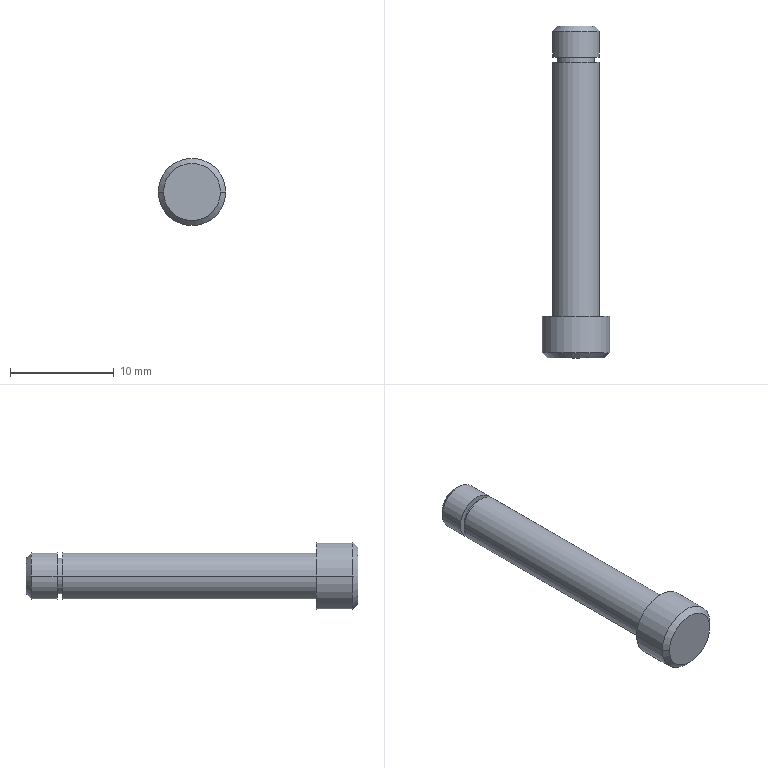Part | Creo | features DATUM PLANE 3, COORDINATE SYSTEM 1, CURVE 1, PROTRUSION 1 | 1 solid | 17 faces | box 6.5 x 32 x 6.5 mm | volume 570.854 mm3 | cylinder 8 | plane 5 | cone 4 | commonest cylinder face diameters 4.5 x4 3.5 x2 6.5 x2
STEP:
#1=CARTESIAN_POINT('',(0.,0.,0.));
#2=DIRECTION('',(0.,0.,1.));
#3=DIRECTION('',(1.,0.,0.));
#4=AXIS2_PLACEMENT_3D('',#1,#2,#3);
#5=CARTESIAN_POINT('',(2.25,4.,0.));
#6=VERTEX_POINT('',#5);
#7=CARTESIAN_POINT('',(2.25,28.5,0.));
#8=VERTEX_POINT('',#7);
#9=CARTESIAN_POINT('',(2.25,4.,0.));
#10=DIRECTION('',(0.,1.,0.));
#11=VECTOR('',#10,24.5);
#12=LINE('',#9,#11);
#13=EDGE_CURVE('',#6,#8,#12,.T.);
#14=ORIENTED_EDGE('',*,*,#13,.T.);
#15=CARTESIAN_POINT('',(-2.25,28.5,0.));
#16=VERTEX_POINT('',#15);
#17=CARTESIAN_POINT('',(0.,28.5,0.));
#18=DIRECTION('',(0.,1.,0.));
#19=DIRECTION('',(1.,0.,0.));
#20=AXIS2_PLACEMENT_3D('',#17,#18,#19);
#21=CIRCLE('',#20,2.25);
#22=EDGE_CURVE('',#8,#16,#21,.T.);
#23=ORIENTED_EDGE('',*,*,#22,.T.);
#24=CARTESIAN_POINT('',(-2.25,4.,0.));
#25=VERTEX_POINT('',#24);
#26=CARTESIAN_POINT('',(-2.25,4.,0.));
#27=DIRECTION('',(0.,1.,0.));
#28=VECTOR('',#27,24.5);
#29=LINE('',#26,#28);
#30=EDGE_CURVE('',#25,#16,#29,.T.);
#31=ORIENTED_EDGE('',*,*,#30,.F.);
#32=CARTESIAN_POINT('',(0.,4.,0.));
#33=DIRECTION('',(0.,1.,0.));
#34=DIRECTION('',(1.,0.,0.));
#35=AXIS2_PLACEMENT_3D('',#32,#33,#34);
#36=CIRCLE('',#35,2.25);
#37=EDGE_CURVE('',#6,#25,#36,.T.);
#38=ORIENTED_EDGE('',*,*,#37,.F.);
#39=EDGE_LOOP('',(#14,#23,#31,#38));
#40=FACE_OUTER_BOUND('',#39,.F.);
#41=CARTESIAN_POINT('',(0.,0.,0.));
#42=DIRECTION('',(0.,1.,0.));
#43=DIRECTION('',(1.,0.,0.));
#44=AXIS2_PLACEMENT_3D('',#41,#42,#43);
#45=CYLINDRICAL_SURFACE('',#44,2.25);
#46=ADVANCED_FACE('',(#40),#45,.T.);
#47=ORIENTED_EDGE('',*,*,#13,.F.);
#48=CARTESIAN_POINT('',(0.,4.,0.));
#49=DIRECTION('',(0.,-1.,0.));
#50=DIRECTION('',(1.,0.,0.));
#51=AXIS2_PLACEMENT_3D('',#48,#49,#50);
#52=CIRCLE('',#51,2.25);
#53=EDGE_CURVE('',#6,#25,#52,.T.);
#54=ORIENTED_EDGE('',*,*,#53,.T.);
#55=ORIENTED_EDGE('',*,*,#30,.T.);
#56=CARTESIAN_POINT('',(0.,28.5,0.));
#57=DIRECTION('',(0.,-1.,0.));
#58=DIRECTION('',(1.,0.,0.));
#59=AXIS2_PLACEMENT_3D('',#56,#57,#58);
#60=CIRCLE('',#59,2.25);
#61=EDGE_CURVE('',#8,#16,#60,.T.);
#62=ORIENTED_EDGE('',*,*,#61,.F.);
#63=EDGE_LOOP('',(#47,#54,#55,#62));
#64=FACE_OUTER_BOUND('',#63,.F.);
#65=CARTESIAN_POINT('',(0.,0.,0.));
#66=DIRECTION('',(0.,1.,0.));
#67=DIRECTION('',(1.,0.,0.));
#68=AXIS2_PLACEMENT_3D('',#65,#66,#67);
#69=CYLINDRICAL_SURFACE('',#68,2.25);
#70=ADVANCED_FACE('',(#64),#69,.T.);
#71=CARTESIAN_POINT('',(3.25,4.,0.));
#72=VERTEX_POINT('',#71);
#73=CARTESIAN_POINT('',(-3.25,4.,0.));
#74=VERTEX_POINT('',#73);
#75=CARTESIAN_POINT('',(0.,4.,0.));
#76=DIRECTION('',(0.,1.,0.));
#77=DIRECTION('',(1.,0.,0.));
#78=AXIS2_PLACEMENT_3D('',#75,#76,#77);
#79=CIRCLE('',#78,3.25);
#80=EDGE_CURVE('',#72,#74,#79,.T.);
#81=ORIENTED_EDGE('',*,*,#80,.F.);
#82=CARTESIAN_POINT('',(0.,4.,0.));
#83=DIRECTION('',(0.,-1.,0.));
#84=DIRECTION('',(1.,0.,0.));
#85=AXIS2_PLACEMENT_3D('',#82,#83,#84);
#86=CIRCLE('',#85,3.25);
#87=EDGE_CURVE('',#72,#74,#86,.T.);
#88=ORIENTED_EDGE('',*,*,#87,.T.);
#89=EDGE_LOOP('',(#81,#88));
#90=FACE_OUTER_BOUND('',#89,.F.);
#91=ORIENTED_EDGE('',*,*,#53,.F.);
#92=ORIENTED_EDGE('',*,*,#37,.T.);
#93=EDGE_LOOP('',(#91,#92));
#94=FACE_BOUND('',#93,.F.);
#95=CARTESIAN_POINT('',(0.,4.,0.));
#96=DIRECTION('',(0.,1.,0.));
#97=DIRECTION('',(1.,0.,0.));
#98=AXIS2_PLACEMENT_3D('',#95,#96,#97);
#99=PLANE('',#98);
#100=ADVANCED_FACE('',(#90,#94),#99,.T.);
#101=CARTESIAN_POINT('',(3.25,0.5,0.));
#102=VERTEX_POINT('',#101);
#103=CARTESIAN_POINT('',(3.25,0.5,0.));
#104=DIRECTION('',(0.,1.,0.));
#105=VECTOR('',#104,3.5);
#106=LINE('',#103,#105);
#107=EDGE_CURVE('',#102,#72,#106,.T.);
#108=ORIENTED_EDGE('',*,*,#107,.T.);
#109=ORIENTED_EDGE('',*,*,#80,.T.);
#110=CARTESIAN_POINT('',(-3.25,0.5,0.));
#111=VERTEX_POINT('',#110);
#112=CARTESIAN_POINT('',(-3.25,0.5,0.));
#113=DIRECTION('',(0.,1.,0.));
#114=VECTOR('',#113,3.5);
#115=LINE('',#112,#114);
#116=EDGE_CURVE('',#111,#74,#115,.T.);
#117=ORIENTED_EDGE('',*,*,#116,.F.);
#118=CARTESIAN_POINT('',(0.,0.5,0.));
#119=DIRECTION('',(0.,1.,0.));
#120=DIRECTION('',(1.,0.,0.));
#121=AXIS2_PLACEMENT_3D('',#118,#119,#120);
#122=CIRCLE('',#121,3.25);
#123=EDGE_CURVE('',#102,#111,#122,.T.);
#124=ORIENTED_EDGE('',*,*,#123,.F.);
#125=EDGE_LOOP('',(#108,#109,#117,#124));
#126=FACE_OUTER_BOUND('',#125,.F.);
#127=CARTESIAN_POINT('',(0.,0.,0.));
#128=DIRECTION('',(0.,1.,0.));
#129=DIRECTION('',(1.,0.,0.));
#130=AXIS2_PLACEMENT_3D('',#127,#128,#129);
#131=CYLINDRICAL_SURFACE('',#130,3.25);
#132=ADVANCED_FACE('',(#126),#131,.T.);
#133=ORIENTED_EDGE('',*,*,#107,.F.);
#134=CARTESIAN_POINT('',(0.,0.5,0.));
#135=DIRECTION('',(0.,-1.,0.));
#136=DIRECTION('',(1.,0.,0.));
#137=AXIS2_PLACEMENT_3D('',#134,#135,#136);
#138=CIRCLE('',#137,3.25);
#139=EDGE_CURVE('',#102,#111,#138,.T.);
#140=ORIENTED_EDGE('',*,*,#139,.T.);
#141=ORIENTED_EDGE('',*,*,#116,.T.);
#142=ORIENTED_EDGE('',*,*,#87,.F.);
#143=EDGE_LOOP('',(#133,#140,#141,#142));
#144=FACE_OUTER_BOUND('',#143,.F.);
#145=CARTESIAN_POINT('',(0.,0.,0.));
#146=DIRECTION('',(0.,1.,0.));
#147=DIRECTION('',(1.,0.,0.));
#148=AXIS2_PLACEMENT_3D('',#145,#146,#147);
#149=CYLINDRICAL_SURFACE('',#148,3.25);
#150=ADVANCED_FACE('',(#144),#149,.T.);
#151=CARTESIAN_POINT('',(2.75,0.,0.));
#152=VERTEX_POINT('',#151);
#153=CARTESIAN_POINT('',(2.75,0.,0.));
#154=DIRECTION('',(0.7071,0.7071,0.));
#155=VECTOR('',#154,0.7071);
#156=LINE('',#153,#155);
#157=EDGE_CURVE('',#152,#102,#156,.T.);
#158=ORIENTED_EDGE('',*,*,#157,.F.);
#159=CARTESIAN_POINT('',(-2.75,0.,0.));
#160=VERTEX_POINT('',#159);
#161=CARTESIAN_POINT('',(0.,0.,0.));
#162=DIRECTION('',(0.,-1.,0.));
#163=DIRECTION('',(1.,0.,0.));
#164=AXIS2_PLACEMENT_3D('',#161,#162,#163);
#165=CIRCLE('',#164,2.75);
#166=EDGE_CURVE('',#152,#160,#165,.T.);
#167=ORIENTED_EDGE('',*,*,#166,.T.);
#168=CARTESIAN_POINT('',(-2.75,0.,0.));
#169=DIRECTION('',(-0.7071,0.7071,0.));
#170=VECTOR('',#169,0.7071);
#171=LINE('',#168,#170);
#172=EDGE_CURVE('',#160,#111,#171,.T.);
#173=ORIENTED_EDGE('',*,*,#172,.T.);
#174=ORIENTED_EDGE('',*,*,#139,.F.);
#175=EDGE_LOOP('',(#158,#167,#173,#174));
#176=FACE_OUTER_BOUND('',#175,.F.);
#177=CARTESIAN_POINT('',(0.,0.25,0.));
#178=DIRECTION('',(0.,1.,0.));
#179=DIRECTION('',(1.,0.,0.));
#180=AXIS2_PLACEMENT_3D('',#177,#178,#179);
#181=CONICAL_SURFACE('',#180,3.,45.);
#182=ADVANCED_FACE('',(#176),#181,.T.);
#183=ORIENTED_EDGE('',*,*,#157,.T.);
#184=ORIENTED_EDGE('',*,*,#123,.T.);
#185=ORIENTED_EDGE('',*,*,#172,.F.);
#186=CARTESIAN_POINT('',(0.,0.,0.));
#187=DIRECTION('',(0.,1.,0.));
#188=DIRECTION('',(1.,0.,0.));
#189=AXIS2_PLACEMENT_3D('',#186,#187,#188);
#190=CIRCLE('',#189,2.75);
#191=EDGE_CURVE('',#152,#160,#190,.T.);
#192=ORIENTED_EDGE('',*,*,#191,.F.);
#193=EDGE_LOOP('',(#183,#184,#185,#192));
#194=FACE_OUTER_BOUND('',#193,.F.);
#195=CARTESIAN_POINT('',(0.,0.25,0.));
#196=DIRECTION('',(0.,1.,0.));
#197=DIRECTION('',(1.,0.,0.));
#198=AXIS2_PLACEMENT_3D('',#195,#196,#197);
#199=CONICAL_SURFACE('',#198,3.,45.);
#200=ADVANCED_FACE('',(#194),#199,.T.);
#201=ORIENTED_EDGE('',*,*,#166,.F.);
#202=ORIENTED_EDGE('',*,*,#191,.T.);
#203=EDGE_LOOP('',(#201,#202));
#204=FACE_OUTER_BOUND('',#203,.F.);
#205=CARTESIAN_POINT('',(0.,0.,0.));
#206=DIRECTION('',(0.,1.,0.));
#207=DIRECTION('',(1.,0.,0.));
#208=AXIS2_PLACEMENT_3D('',#205,#206,#207);
#209=PLANE('',#208);
#210=ADVANCED_FACE('',(#204),#209,.F.);
#211=ORIENTED_EDGE('',*,*,#61,.T.);
#212=ORIENTED_EDGE('',*,*,#22,.F.);
#213=EDGE_LOOP('',(#211,#212));
#214=FACE_OUTER_BOUND('',#213,.F.);
#215=CARTESIAN_POINT('',(1.75,28.5,0.));
#216=VERTEX_POINT('',#215);
#217=CARTESIAN_POINT('',(-1.75,28.5,0.));
#218=VERTEX_POINT('',#217);
#219=CARTESIAN_POINT('',(0.,28.5,0.));
#220=DIRECTION('',(0.,1.,0.));
#221=DIRECTION('',(1.,0.,0.));
#222=AXIS2_PLACEMENT_3D('',#219,#220,#221);
#223=CIRCLE('',#222,1.75);
#224=EDGE_CURVE('',#216,#218,#223,.T.);
#225=ORIENTED_EDGE('',*,*,#224,.T.);
#226=CARTESIAN_POINT('',(0.,28.5,0.));
#227=DIRECTION('',(0.,-1.,0.));
#228=DIRECTION('',(1.,0.,0.));
#229=AXIS2_PLACEMENT_3D('',#226,#227,#228);
#230=CIRCLE('',#229,1.75);
#231=EDGE_CURVE('',#216,#218,#230,.T.);
#232=ORIENTED_EDGE('',*,*,#231,.F.);
#233=EDGE_LOOP('',(#225,#232));
#234=FACE_BOUND('',#233,.F.);
#235=CARTESIAN_POINT('',(0.,28.5,0.));
#236=DIRECTION('',(0.,1.,0.));
#237=DIRECTION('',(1.,0.,0.));
#238=AXIS2_PLACEMENT_3D('',#235,#236,#237);
#239=PLANE('',#238);
#240=ADVANCED_FACE('',(#214,#234),#239,.T.);
#241=CARTESIAN_POINT('',(1.75,29.,0.));
#242=VERTEX_POINT('',#241);
#243=CARTESIAN_POINT('',(1.75,28.5,0.));
#244=DIRECTION('',(0.,1.,0.));
#245=VECTOR('',#244,0.5);
#246=LINE('',#243,#245);
#247=EDGE_CURVE('',#216,#242,#246,.T.);
#248=ORIENTED_EDGE('',*,*,#247,.T.);
#249=CARTESIAN_POINT('',(-1.75,29.,0.));
#250=VERTEX_POINT('',#249);
#251=CARTESIAN_POINT('',(0.,29.,0.));
#252=DIRECTION('',(0.,1.,0.));
#253=DIRECTION('',(1.,0.,0.));
#254=AXIS2_PLACEMENT_3D('',#251,#252,#253);
#255=CIRCLE('',#254,1.75);
#256=EDGE_CURVE('',#242,#250,#255,.T.);
#257=ORIENTED_EDGE('',*,*,#256,.T.);
#258=CARTESIAN_POINT('',(-1.75,28.5,0.));
#259=DIRECTION('',(0.,1.,0.));
#260=VECTOR('',#259,0.5);
#261=LINE('',#258,#260);
#262=EDGE_CURVE('',#218,#250,#261,.T.);
#263=ORIENTED_EDGE('',*,*,#262,.F.);
#264=ORIENTED_EDGE('',*,*,#224,.F.);
#265=EDGE_LOOP('',(#248,#257,#263,#264));
#266=FACE_OUTER_BOUND('',#265,.F.);
#267=CARTESIAN_POINT('',(0.,0.,0.));
#268=DIRECTION('',(0.,1.,0.));
#269=DIRECTION('',(1.,0.,0.));
#270=AXIS2_PLACEMENT_3D('',#267,#268,#269);
#271=CYLINDRICAL_SURFACE('',#270,1.75);
#272=ADVANCED_FACE('',(#266),#271,.T.);
#273=ORIENTED_EDGE('',*,*,#247,.F.);
#274=ORIENTED_EDGE('',*,*,#231,.T.);
#275=ORIENTED_EDGE('',*,*,#262,.T.);
#276=CARTESIAN_POINT('',(0.,29.,0.));
#277=DIRECTION('',(0.,-1.,0.));
#278=DIRECTION('',(1.,0.,0.));
#279=AXIS2_PLACEMENT_3D('',#276,#277,#278);
#280=CIRCLE('',#279,1.75);
#281=EDGE_CURVE('',#242,#250,#280,.T.);
#282=ORIENTED_EDGE('',*,*,#281,.F.);
#283=EDGE_LOOP('',(#273,#274,#275,#282));
#284=FACE_OUTER_BOUND('',#283,.F.);
#285=CARTESIAN_POINT('',(0.,0.,0.));
#286=DIRECTION('',(0.,1.,0.));
#287=DIRECTION('',(1.,0.,0.));
#288=AXIS2_PLACEMENT_3D('',#285,#286,#287);
#289=CYLINDRICAL_SURFACE('',#288,1.75);
#290=ADVANCED_FACE('',(#284),#289,.T.);
#291=CARTESIAN_POINT('',(2.25,29.,0.));
#292=VERTEX_POINT('',#291);
#293=CARTESIAN_POINT('',(-2.25,29.,0.));
#294=VERTEX_POINT('',#293);
#295=CARTESIAN_POINT('',(0.,29.,0.));
#296=DIRECTION('',(0.,1.,0.));
#297=DIRECTION('',(1.,0.,0.));
#298=AXIS2_PLACEMENT_3D('',#295,#296,#297);
#299=CIRCLE('',#298,2.25);
#300=EDGE_CURVE('',#292,#294,#299,.T.);
#301=ORIENTED_EDGE('',*,*,#300,.T.);
#302=CARTESIAN_POINT('',(0.,29.,0.));
#303=DIRECTION('',(0.,-1.,0.));
#304=DIRECTION('',(1.,0.,0.));
#305=AXIS2_PLACEMENT_3D('',#302,#303,#304);
#306=CIRCLE('',#305,2.25);
#307=EDGE_CURVE('',#292,#294,#306,.T.);
#308=ORIENTED_EDGE('',*,*,#307,.F.);
#309=EDGE_LOOP('',(#301,#308));
#310=FACE_OUTER_BOUND('',#309,.F.);
#311=ORIENTED_EDGE('',*,*,#281,.T.);
#312=ORIENTED_EDGE('',*,*,#256,.F.);
#313=EDGE_LOOP('',(#311,#312));
#314=FACE_BOUND('',#313,.F.);
#315=CARTESIAN_POINT('',(0.,29.,0.));
#316=DIRECTION('',(0.,1.,0.));
#317=DIRECTION('',(1.,0.,0.));
#318=AXIS2_PLACEMENT_3D('',#315,#316,#317);
#319=PLANE('',#318);
#320=ADVANCED_FACE('',(#310,#314),#319,.F.);
#321=CARTESIAN_POINT('',(2.25,31.5,0.));
#322=VERTEX_POINT('',#321);
#323=CARTESIAN_POINT('',(2.25,29.,0.));
#324=DIRECTION('',(0.,1.,0.));
#325=VECTOR('',#324,2.5);
#326=LINE('',#323,#325);
#327=EDGE_CURVE('',#292,#322,#326,.T.);
#328=ORIENTED_EDGE('',*,*,#327,.T.);
#329=CARTESIAN_POINT('',(-2.25,31.5,0.));
#330=VERTEX_POINT('',#329);
#331=CARTESIAN_POINT('',(0.,31.5,0.));
#332=DIRECTION('',(0.,1.,0.));
#333=DIRECTION('',(1.,0.,0.));
#334=AXIS2_PLACEMENT_3D('',#331,#332,#333);
#335=CIRCLE('',#334,2.25);
#336=EDGE_CURVE('',#322,#330,#335,.T.);
#337=ORIENTED_EDGE('',*,*,#336,.T.);
#338=CARTESIAN_POINT('',(-2.25,29.,0.));
#339=DIRECTION('',(0.,1.,0.));
#340=VECTOR('',#339,2.5);
#341=LINE('',#338,#340);
#342=EDGE_CURVE('',#294,#330,#341,.T.);
#343=ORIENTED_EDGE('',*,*,#342,.F.);
#344=ORIENTED_EDGE('',*,*,#300,.F.);
#345=EDGE_LOOP('',(#328,#337,#343,#344));
#346=FACE_OUTER_BOUND('',#345,.F.);
#347=CARTESIAN_POINT('',(0.,0.,0.));
#348=DIRECTION('',(0.,1.,0.));
#349=DIRECTION('',(1.,0.,0.));
#350=AXIS2_PLACEMENT_3D('',#347,#348,#349);
#351=CYLINDRICAL_SURFACE('',#350,2.25);
#352=ADVANCED_FACE('',(#346),#351,.T.);
#353=ORIENTED_EDGE('',*,*,#327,.F.);
#354=ORIENTED_EDGE('',*,*,#307,.T.);
#355=ORIENTED_EDGE('',*,*,#342,.T.);
#356=CARTESIAN_POINT('',(0.,31.5,0.));
#357=DIRECTION('',(0.,-1.,0.));
#358=DIRECTION('',(1.,0.,0.));
#359=AXIS2_PLACEMENT_3D('',#356,#357,#358);
#360=CIRCLE('',#359,2.25);
#361=EDGE_CURVE('',#322,#330,#360,.T.);
#362=ORIENTED_EDGE('',*,*,#361,.F.);
#363=EDGE_LOOP('',(#353,#354,#355,#362));
#364=FACE_OUTER_BOUND('',#363,.F.);
#365=CARTESIAN_POINT('',(0.,0.,0.));
#366=DIRECTION('',(0.,1.,0.));
#367=DIRECTION('',(1.,0.,0.));
#368=AXIS2_PLACEMENT_3D('',#365,#366,#367);
#369=CYLINDRICAL_SURFACE('',#368,2.25);
#370=ADVANCED_FACE('',(#364),#369,.T.);
#371=CARTESIAN_POINT('',(1.75,32.,0.));
#372=VERTEX_POINT('',#371);
#373=CARTESIAN_POINT('',(2.25,31.5,0.));
#374=DIRECTION('',(-0.7071,0.7071,0.));
#375=VECTOR('',#374,0.7071);
#376=LINE('',#373,#375);
#377=EDGE_CURVE('',#322,#372,#376,.T.);
#378=ORIENTED_EDGE('',*,*,#377,.F.);
#379=ORIENTED_EDGE('',*,*,#361,.T.);
#380=CARTESIAN_POINT('',(-1.75,32.,0.));
#381=VERTEX_POINT('',#380);
#382=CARTESIAN_POINT('',(-2.25,31.5,0.));
#383=DIRECTION('',(0.7071,0.7071,0.));
#384=VECTOR('',#383,0.7071);
#385=LINE('',#382,#384);
#386=EDGE_CURVE('',#330,#381,#385,.T.);
#387=ORIENTED_EDGE('',*,*,#386,.T.);
#388=CARTESIAN_POINT('',(0.,32.,0.));
#389=DIRECTION('',(0.,-1.,0.));
#390=DIRECTION('',(1.,0.,0.));
#391=AXIS2_PLACEMENT_3D('',#388,#389,#390);
#392=CIRCLE('',#391,1.75);
#393=EDGE_CURVE('',#372,#381,#392,.T.);
#394=ORIENTED_EDGE('',*,*,#393,.F.);
#395=EDGE_LOOP('',(#378,#379,#387,#394));
#396=FACE_OUTER_BOUND('',#395,.F.);
#397=CARTESIAN_POINT('',(0.,31.75,0.));
#398=DIRECTION('',(0.,-1.,0.));
#399=DIRECTION('',(-1.,0.,0.));
#400=AXIS2_PLACEMENT_3D('',#397,#398,#399);
#401=CONICAL_SURFACE('',#400,2.,45.);
#402=ADVANCED_FACE('',(#396),#401,.T.);
#403=ORIENTED_EDGE('',*,*,#377,.T.);
#404=CARTESIAN_POINT('',(0.,32.,0.));
#405=DIRECTION('',(0.,1.,0.));
#406=DIRECTION('',(1.,0.,0.));
#407=AXIS2_PLACEMENT_3D('',#404,#405,#406);
#408=CIRCLE('',#407,1.75);
#409=EDGE_CURVE('',#372,#381,#408,.T.);
#410=ORIENTED_EDGE('',*,*,#409,.T.);
#411=ORIENTED_EDGE('',*,*,#386,.F.);
#412=ORIENTED_EDGE('',*,*,#336,.F.);
#413=EDGE_LOOP('',(#403,#410,#411,#412));
#414=FACE_OUTER_BOUND('',#413,.F.);
#415=CARTESIAN_POINT('',(0.,31.75,0.));
#416=DIRECTION('',(0.,-1.,0.));
#417=DIRECTION('',(-1.,0.,0.));
#418=AXIS2_PLACEMENT_3D('',#415,#416,#417);
#419=CONICAL_SURFACE('',#418,2.,45.);
#420=ADVANCED_FACE('',(#414),#419,.T.);
#421=ORIENTED_EDGE('',*,*,#393,.T.);
#422=ORIENTED_EDGE('',*,*,#409,.F.);
#423=EDGE_LOOP('',(#421,#422));
#424=FACE_OUTER_BOUND('',#423,.F.);
#425=CARTESIAN_POINT('',(0.,32.,0.));
#426=DIRECTION('',(0.,1.,0.));
#427=DIRECTION('',(1.,0.,0.));
#428=AXIS2_PLACEMENT_3D('',#425,#426,#427);
#429=PLANE('',#428);
#430=ADVANCED_FACE('',(#424),#429,.T.);
#431=CLOSED_SHELL('',(#46,#70,#100,#132,#150,#182,#200,#210,#240,#272,#290,#320,#352,#370,#402,#420,#430));
#432=MANIFOLD_SOLID_BREP('',#431);
#433=(LENGTH_UNIT()NAMED_UNIT(*)SI_UNIT(.MILLI.,.METRE.));
#434=UNCERTAINTY_MEASURE_WITH_UNIT(LENGTH_MEASURE(0.003329),#433,'','');
#435=(NAMED_UNIT(*)PLANE_ANGLE_UNIT()SI_UNIT($,.RADIAN.));
#436=PLANE_ANGLE_MEASURE_WITH_UNIT(PLANE_ANGLE_MEASURE(0.01745),#435);
#437=(CONVERSION_BASED_UNIT('DEGREE',#436)NAMED_UNIT(*)PLANE_ANGLE_UNIT());
#438=(NAMED_UNIT(*)SI_UNIT($,.STERADIAN.)SOLID_ANGLE_UNIT());
#439=(GEOMETRIC_REPRESENTATION_CONTEXT(3)GLOBAL_UNCERTAINTY_ASSIGNED_CONTEXT((#434))GLOBAL_UNIT_ASSIGNED_CONTEXT((#433,#437,#438))REPRESENTATION_CONTEXT('',''));
#440=ADVANCED_BREP_SHAPE_REPRESENTATION('',(#4,#432),#439);